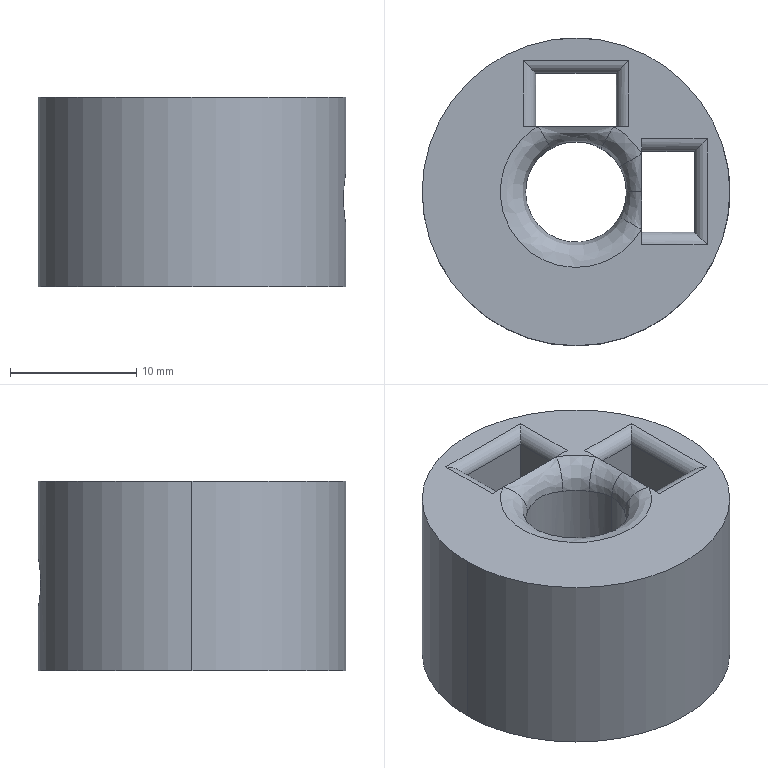Part | SolidWorks | features BaseBody 1 | 1 solid | 37 faces | box 24.4 x 24.4 x 15 mm | volume 5383 mm3 | cylinder 18 | plane 10 | spline 9 | commonest cylinder face diameters 2.4 x8 2 x6 8 x2 24.4 x2